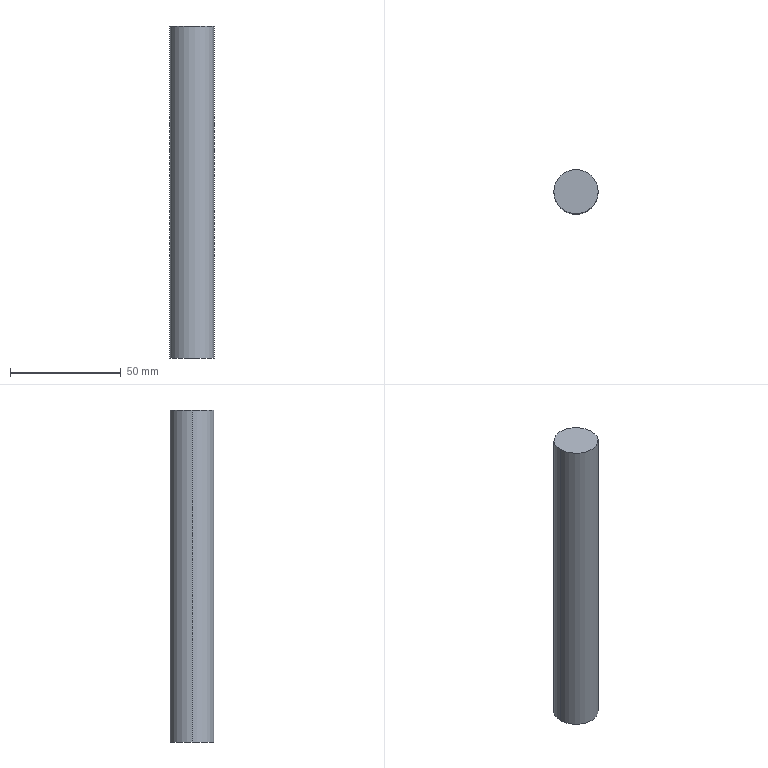Part | SolidWorks | features Extrusion 1 | 1 solid | 4 faces | box 20 x 20 x 150 mm | volume 47124 mm3 | cylinder 2 | plane 2 | commonest cylinder face diameters 20 x2
STEP:
#1=CARTESIAN_POINT('',(10.,0.,150.));
#2=VERTEX_POINT('',#1);
#3=CARTESIAN_POINT('',(-10.,0.,150.));
#4=VERTEX_POINT('',#3);
#5=CARTESIAN_POINT('',(0.,0.,150.));
#6=DIRECTION('',(0.,0.,1.));
#7=DIRECTION('',(1.,0.,0.));
#8=AXIS2_PLACEMENT_3D('',#5,#6,#7);
#9=CIRCLE('',#8,10.);
#10=EDGE_CURVE('',#2,#4,#9,.T.);
#11=ORIENTED_EDGE('',*,*,#10,.F.);
#12=CARTESIAN_POINT('',(10.,0.,0.));
#13=VERTEX_POINT('',#12);
#14=CARTESIAN_POINT('',(10.,0.,150.));
#15=DIRECTION('',(0.,0.,-1.));
#16=VECTOR('',#15,1000.);
#17=LINE('',#14,#16);
#18=EDGE_CURVE('',#2,#13,#17,.T.);
#19=ORIENTED_EDGE('',*,*,#18,.T.);
#20=CARTESIAN_POINT('',(-10.,0.,0.));
#21=VERTEX_POINT('',#20);
#22=CARTESIAN_POINT('',(0.,0.,0.));
#23=DIRECTION('',(0.,0.,1.));
#24=DIRECTION('',(1.,0.,0.));
#25=AXIS2_PLACEMENT_3D('',#22,#23,#24);
#26=CIRCLE('',#25,10.);
#27=EDGE_CURVE('',#13,#21,#26,.T.);
#28=ORIENTED_EDGE('',*,*,#27,.T.);
#29=CARTESIAN_POINT('',(-10.,0.,150.));
#30=DIRECTION('',(0.,0.,-1.));
#31=VECTOR('',#30,1000.);
#32=LINE('',#29,#31);
#33=EDGE_CURVE('',#4,#21,#32,.T.);
#34=ORIENTED_EDGE('',*,*,#33,.F.);
#35=EDGE_LOOP('',(#11,#19,#28,#34));
#36=FACE_OUTER_BOUND('',#35,.T.);
#37=CARTESIAN_POINT('',(0.,0.,150.));
#38=DIRECTION('',(0.,0.,-1.));
#39=DIRECTION('',(-1.,0.,0.));
#40=AXIS2_PLACEMENT_3D('',#37,#38,#39);
#41=CYLINDRICAL_SURFACE('',#40,10.);
#42=ADVANCED_FACE('',(#36),#41,.T.);
#43=ORIENTED_EDGE('',*,*,#18,.F.);
#44=CARTESIAN_POINT('',(0.,0.,150.));
#45=DIRECTION('',(0.,0.,1.));
#46=DIRECTION('',(1.,0.,0.));
#47=AXIS2_PLACEMENT_3D('',#44,#45,#46);
#48=CIRCLE('',#47,10.);
#49=EDGE_CURVE('',#4,#2,#48,.T.);
#50=ORIENTED_EDGE('',*,*,#49,.F.);
#51=ORIENTED_EDGE('',*,*,#33,.T.);
#52=CARTESIAN_POINT('',(0.,0.,0.));
#53=DIRECTION('',(0.,0.,1.));
#54=DIRECTION('',(1.,0.,0.));
#55=AXIS2_PLACEMENT_3D('',#52,#53,#54);
#56=CIRCLE('',#55,10.);
#57=EDGE_CURVE('',#21,#13,#56,.T.);
#58=ORIENTED_EDGE('',*,*,#57,.T.);
#59=EDGE_LOOP('',(#43,#50,#51,#58));
#60=FACE_OUTER_BOUND('',#59,.T.);
#61=CARTESIAN_POINT('',(0.,0.,150.));
#62=DIRECTION('',(0.,0.,-1.));
#63=DIRECTION('',(-1.,0.,0.));
#64=AXIS2_PLACEMENT_3D('',#61,#62,#63);
#65=CYLINDRICAL_SURFACE('',#64,10.);
#66=ADVANCED_FACE('',(#60),#65,.T.);
#67=ORIENTED_EDGE('',*,*,#49,.T.);
#68=ORIENTED_EDGE('',*,*,#10,.T.);
#69=EDGE_LOOP('',(#67,#68));
#70=FACE_OUTER_BOUND('',#69,.T.);
#71=CARTESIAN_POINT('',(0.,0.,150.));
#72=DIRECTION('',(0.,0.,1.));
#73=DIRECTION('',(1.,0.,0.));
#74=AXIS2_PLACEMENT_3D('',#71,#72,#73);
#75=PLANE('',#74);
#76=ADVANCED_FACE('',(#70),#75,.T.);
#77=ORIENTED_EDGE('',*,*,#57,.F.);
#78=ORIENTED_EDGE('',*,*,#27,.F.);
#79=EDGE_LOOP('',(#77,#78));
#80=FACE_OUTER_BOUND('',#79,.T.);
#81=CARTESIAN_POINT('',(0.,0.,0.));
#82=DIRECTION('',(0.,0.,1.));
#83=DIRECTION('',(1.,0.,0.));
#84=AXIS2_PLACEMENT_3D('',#81,#82,#83);
#85=PLANE('',#84);
#86=ADVANCED_FACE('',(#80),#85,.F.);
#87=CLOSED_SHELL('',(#42,#66,#76,#86));
#88=MANIFOLD_SOLID_BREP('',#87);
#89=CARTESIAN_POINT('',(0.,0.,0.));
#90=DIRECTION('',(0.,0.,1.));
#91=DIRECTION('',(1.,0.,0.));
#92=AXIS2_PLACEMENT_3D('',#89,#90,#91);
#93=(LENGTH_UNIT()NAMED_UNIT(*)SI_UNIT(.MILLI.,.METRE.));
#94=UNCERTAINTY_MEASURE_WITH_UNIT(LENGTH_MEASURE(0.00001),#93,'','');
#95=(NAMED_UNIT(*)PLANE_ANGLE_UNIT()SI_UNIT($,.RADIAN.));
#96=(NAMED_UNIT(*)SI_UNIT($,.STERADIAN.)SOLID_ANGLE_UNIT());
#97=(GEOMETRIC_REPRESENTATION_CONTEXT(3)GLOBAL_UNCERTAINTY_ASSIGNED_CONTEXT((#94))GLOBAL_UNIT_ASSIGNED_CONTEXT((#93,#95,#96))REPRESENTATION_CONTEXT('',''));
#98=ADVANCED_BREP_SHAPE_REPRESENTATION('',(#88,#92),#97);